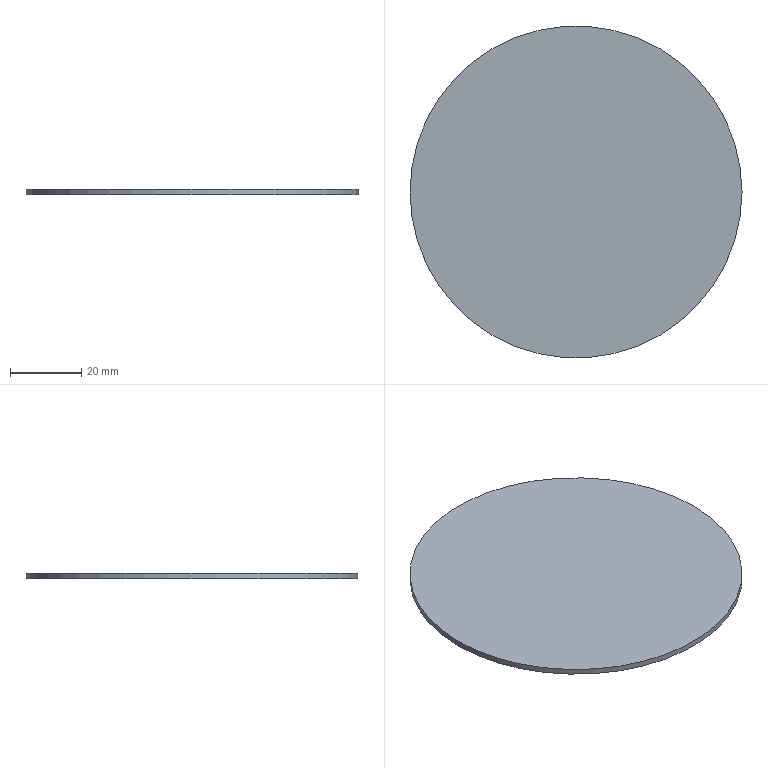Part | NX | features solid 2 | 1 solid | 3 faces | box 93.2 x 93.2 x 1.6 mm | volume 10915 mm3 | plane 2 | cylinder 1 | commonest cylinder face diameters 93.2 x1
STEP:
#1=CARTESIAN_POINT('',(-1246.6,525.,-195.));
#2=VERTEX_POINT('',#1);
#3=CARTESIAN_POINT('',(-1200.,525.,-195.));
#4=DIRECTION('',(0.,0.,1.));
#5=DIRECTION('',(-1.,0.,0.));
#6=AXIS2_PLACEMENT_3D('',#3,#4,#5);
#7=CIRCLE('',#6,46.6);
#8=EDGE_CURVE('',#2,#2,#7,.T.);
#9=ORIENTED_EDGE('',*,*,#8,.T.);
#10=EDGE_LOOP('',(#9));
#11=FACE_BOUND('',#10,.T.);
#12=CARTESIAN_POINT('',(-1246.6,525.,-193.4));
#13=VERTEX_POINT('',#12);
#14=CARTESIAN_POINT('',(-1200.,525.,-193.4));
#15=DIRECTION('',(0.,0.,1.));
#16=DIRECTION('',(-1.,0.,0.));
#17=AXIS2_PLACEMENT_3D('',#14,#15,#16);
#18=CIRCLE('',#17,46.6);
#19=EDGE_CURVE('',#13,#13,#18,.T.);
#20=ORIENTED_EDGE('',*,*,#19,.F.);
#21=EDGE_LOOP('',(#20));
#22=FACE_BOUND('',#21,.T.);
#23=CARTESIAN_POINT('',(-1200.,525.,-195.));
#24=DIRECTION('',(0.,0.,1.));
#25=DIRECTION('',(-1.,0.,0.));
#26=AXIS2_PLACEMENT_3D('',#23,#24,#25);
#27=CYLINDRICAL_SURFACE('',#26,46.6);
#28=ADVANCED_FACE('',(#11,#22),#27,.T.);
#29=ORIENTED_EDGE('',*,*,#8,.F.);
#30=EDGE_LOOP('',(#29));
#31=FACE_BOUND('',#30,.T.);
#32=CARTESIAN_POINT('',(-1200.,525.,-195.));
#33=DIRECTION('',(0.,0.,1.));
#34=DIRECTION('',(-1.,0.,0.));
#35=AXIS2_PLACEMENT_3D('',#32,#33,#34);
#36=PLANE('',#35);
#37=ADVANCED_FACE('',(#31),#36,.F.);
#38=ORIENTED_EDGE('',*,*,#19,.T.);
#39=EDGE_LOOP('',(#38));
#40=FACE_BOUND('',#39,.T.);
#41=CARTESIAN_POINT('',(-1200.,525.,-193.4));
#42=DIRECTION('',(0.,0.,1.));
#43=DIRECTION('',(-1.,0.,0.));
#44=AXIS2_PLACEMENT_3D('',#41,#42,#43);
#45=PLANE('',#44);
#46=ADVANCED_FACE('',(#40),#45,.T.);
#47=CLOSED_SHELL('',(#28,#37,#46));
#48=MANIFOLD_SOLID_BREP('',#47);
#49=(LENGTH_UNIT()NAMED_UNIT(*)SI_UNIT(.MILLI.,.METRE.));
#50=UNCERTAINTY_MEASURE_WITH_UNIT(LENGTH_MEASURE(0.00001),#49,'','');
#51=(NAMED_UNIT(*)PLANE_ANGLE_UNIT()SI_UNIT($,.RADIAN.));
#52=(NAMED_UNIT(*)SI_UNIT($,.STERADIAN.)SOLID_ANGLE_UNIT());
#53=(GEOMETRIC_REPRESENTATION_CONTEXT(3)GLOBAL_UNCERTAINTY_ASSIGNED_CONTEXT((#50))GLOBAL_UNIT_ASSIGNED_CONTEXT((#49,#51,#52))REPRESENTATION_CONTEXT('',''));
#54=ADVANCED_BREP_SHAPE_REPRESENTATION('',(#48),#53);